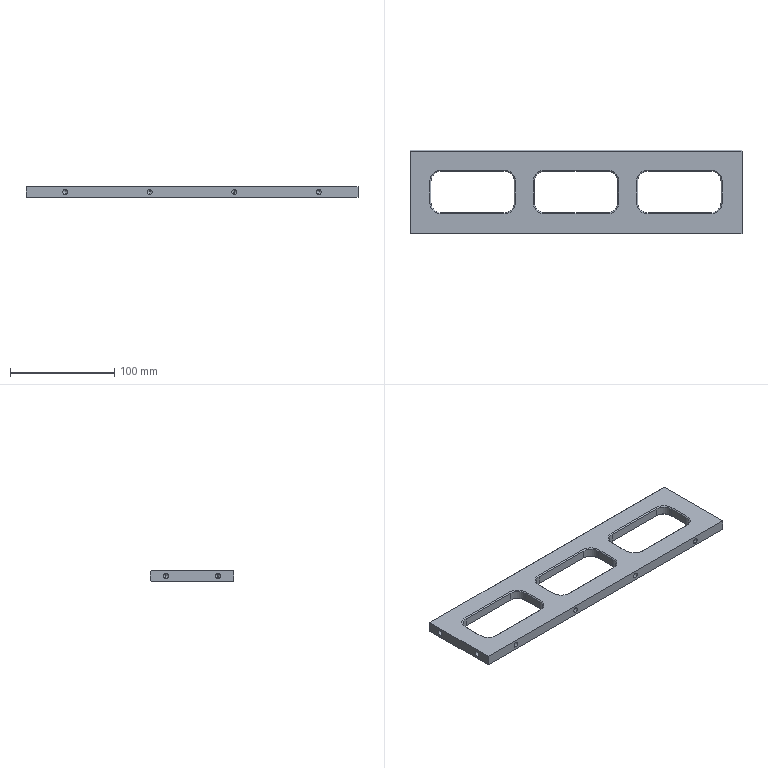Part | SolidWorks | features HoleWzd 3, ICE 3, Chamfer 1, Extrusion 1, Fillet 1 | 1 solid | 112 faces | box 318 x 80 x 10 mm | volume 157548 mm3 | plane 44 | cone 40 | cylinder 28 | commonest cylinder face diameters 5 x16 20 x12